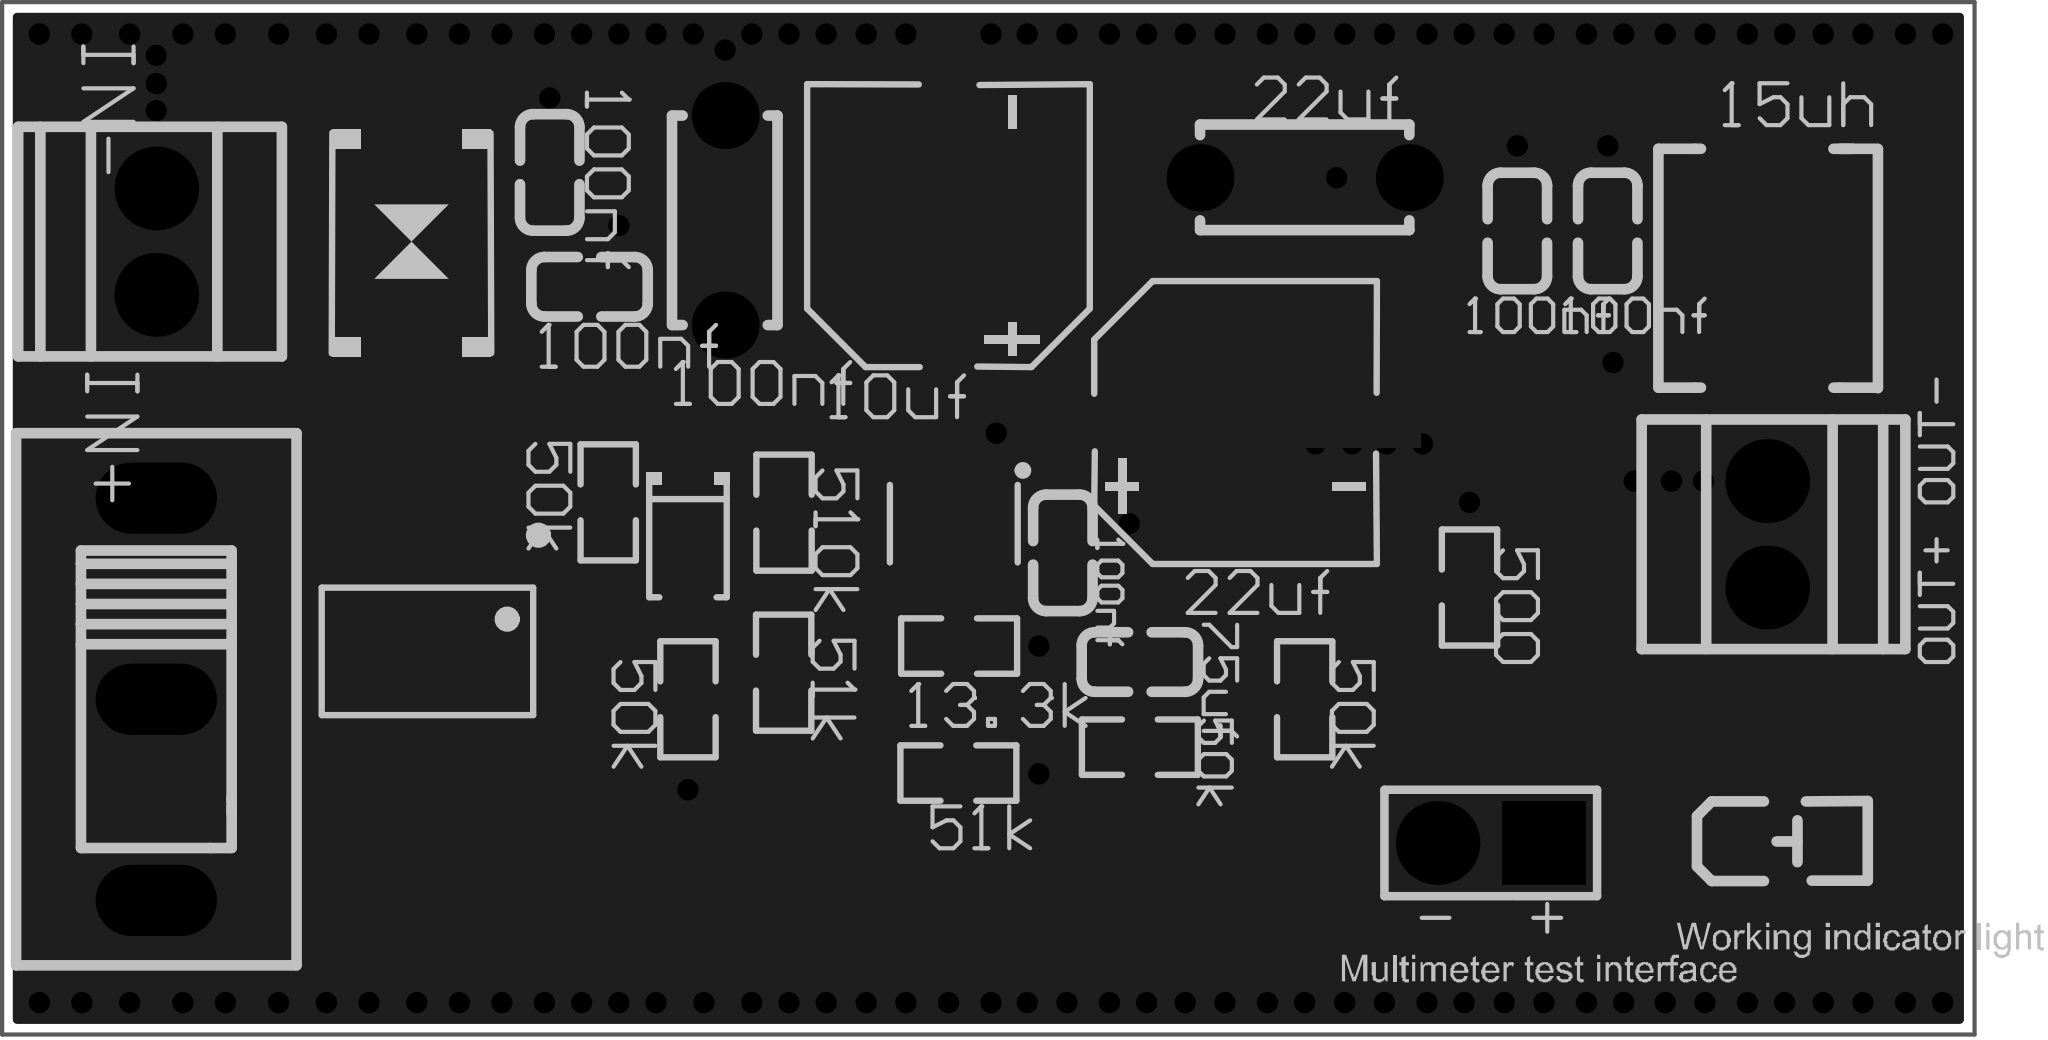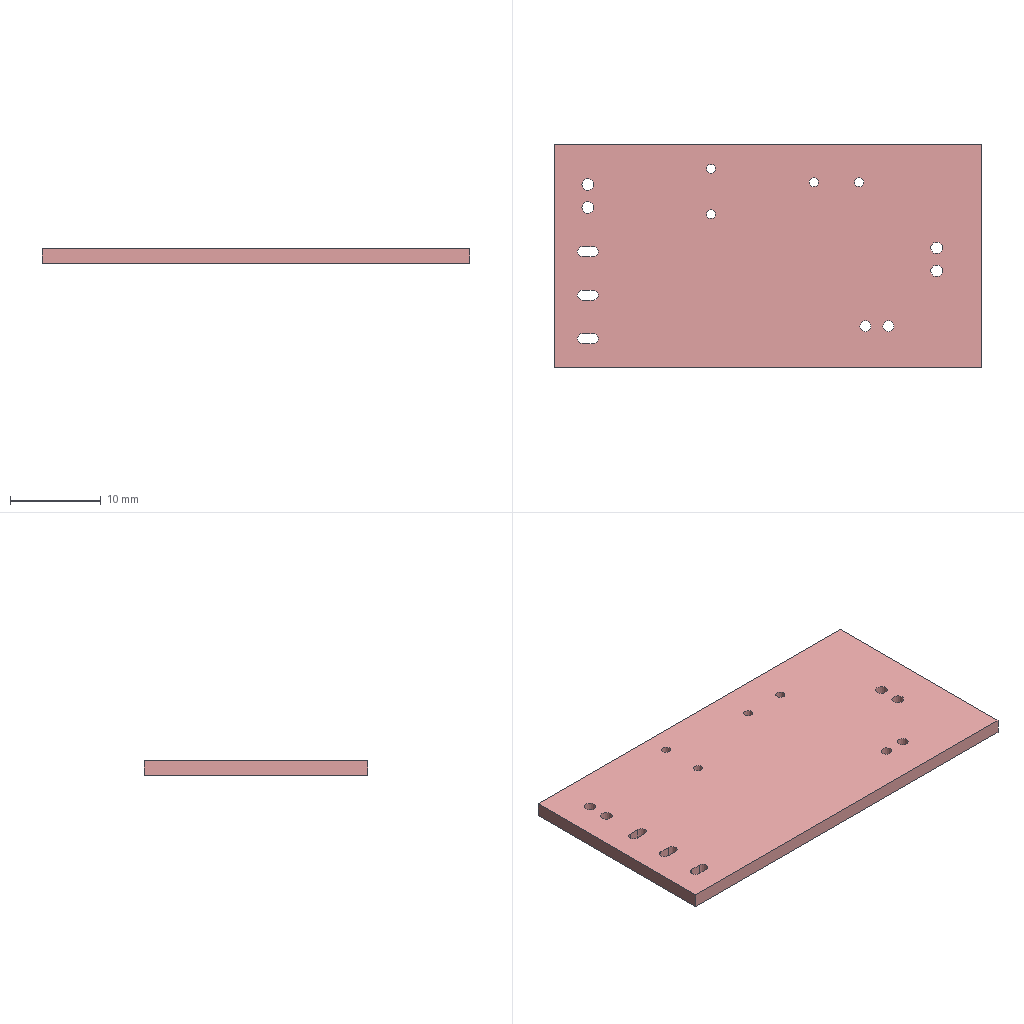Circuit board layout | Altium Designer | box 47.1 x 24.6 x 1.6 mm
Layer stack:
# Altium Designer layer stack of  (unit mm; dielectric type: 0 none, 1 core, 2 prepreg, 3 surface material)
index,name,kind,layer,copper_thickness_mm,dielectric_type,dielectric_thickness_mm,dielectric_material,dielectric_constant
0,Top Paste Mask Layer,other,,,,,,
1,Top Silkscreen Layer,other,,,,,,
2,Top Solder Mask Layer,dielectric,,,3,0.01,,3.3
3,Top Layer,copper,Top Layer,0.035,,,,
4,Dielectric1,dielectric,,,3,1.51,FR4,4.5
5,Bottom Layer,copper,Bottom Layer,0.035,,,,
6,Bottom Solder Mask Layer,dielectric,,,3,0.01,,3.3
7,Bottom Silkscreen Layer,other,,,,,,
8,Bottom Paste Mask Layer,other,,,,,,
# drill layer pairs: low layer,high layer
drill_pair,Top Layer,Bottom Layer
Part placement:
Designator,Comment,Layer,Footprint,Center-X(mm),Center-Y(mm),Rotation
C1,75uf,TopLayer,C0603,107.569,92.71,0
C5,0.1uf,TopLayer,C0603,105.729,95.315,270
C11,10uf,TopLayer,CAP-SMD_BD6.3-L6.6-W6.6-FD,102.997,103.124,90
C12,100nf,TopLayer,CAP-TH_L5.0-W2.5-P5.00-D1.0,97.663,103.251,270
C13,22uf,TopLayer,CAP-SMD_BD6.3-L6.6-W6.6-FD,109.855,98.425,0
C16,22uf,TopLayer,CAP-TH_L5.0-W2.5-P5.00-D1.0,111.506,104.267,180
D3,SMBJ28CA,TopLayer,SMB_L4.6-W3.6-LS5.4-BI,90.17,102.743,270
D4,BZT52C12,TopLayer,SOD-123_L2.7-W1.6-LS3.7-RD,96.774,95.631,270
H3,PZ254V-11-02P,TopLayer,HDR-TH_2P-P2.54-V-M,115.951,88.392,180
L1,15uH,TopLayer,IND-SMD_L5.7-W5.2_GSM0530,122.555,102.108,90
LED1,NCD0805R1,TopLayer,LED0805-RD,122.977,88.433,0
Q1,AO4421,TopLayer,SOIC-8_L4.9-W3.9-P1.27-LS6.0-BL,90.551,92.964,180
SW1,SS12D10G4 071,TopLayer,SW-TH_SHOU-HAN_SS12D10G4,84.074,91.821,270
U1,GD30DC1354,TopLayer,SOT-23-6_L2.9-W1.7-P0.95-LS2.8-BL,103.124,96.012,180
U2,KF128-2.54-2P,TopLayer,CONN-TH_P2.54_KF128-2.54-2P,122.555,95.758,90
U3,KF128-2.54-2P,TopLayer,CONN-TH_P2.54_KF128-2.54-2P,84.074,102.743,270
C21,0.1uf,TopLayer,C0603,118.745,102.997,90
C22,0.1uf,TopLayer,C0603,116.586,102.997,90
C23,100nf,TopLayer,C0603,94.423,101.665,0
C24,100nf,TopLayer,C0603,93.472,104.394,90
R7,510kΩ,TopLayer,R0603,99.069,96.275,90
R8,51kΩ,TopLayer,R0603,99.06,92.456,90
R9,500Ω,TopLayer,R0603,115.443,94.488,270
R10,50kΩ,TopLayer,R0603,107.569,90.678,0
R11,13.3kΩ,TopLayer,R0603,103.251,93.091,180
R12,50kΩ,TopLayer,R0603,111.506,91.821,90
R13,51kΩ,TopLayer,R0603,103.234,90.06,180
R15,50kΩ,TopLayer,R0603,96.774,91.821,90
R16,50kΩ,TopLayer,R0603,94.869,96.52,90
Pad and via stacks:
# Altium Designer via and pad stacks of  (unit mm). Each distinct definition once, with the count of objects using it.
# via: kind,start_layer,end_layer,hole_mm,diameter_mm,mode(0 simple;1 top-mid-bottom;2 full stack),diameter_per_layer,count,example_net
# pad: kind,layer,hole_mm,hole_type(0 round;1 square;2 slot),plating,top_size,top_shape(1 round;2 rect;3 octagon;9 rounded rect),mid_size,bottom_size,mode,footprint,size_per_layer,count,example
pad,Top Layer,0,0,plated,0.8x0.9,2,0.8x0.9,0.8x0.9,0,C0603,,12,C1.2
pad,Top Layer,0,0,plated,3.5x1.2,2,3.5x1.2,3.5x1.2,0,CAP-SMD_BD6.3-L6.6-W6.6-FD,,4,C11.1
pad,Top Layer,0,0,plated,2.047x2.241,2,2.047x2.241,2.047x2.241,0,SMB_L4.6-W3.6-LS5.4-BI,,2,D3.2
pad,Top Layer,0,0,plated,0.91x1.22,2,0.91x1.22,0.91x1.22,0,SOD-123_L2.7-W1.6-LS3.7-RD,,2,D4.2
pad,Top Layer,0,0,plated,1.5x2.7,2,1.5x2.7,1.5x2.7,0,IND-SMD_L5.7-W5.2_GSM0530,,2,L1.2
pad,Top Layer,0,0,plated,1x1.25,2,1x1.25,1x1.25,0,LED0805-RD,,2,LED1.2
pad,Top Layer,0,0,plated,0.588x2.045,1,0.588x2.045,0.588x2.045,0,SOIC-8_L4.9-W3.9-P1.27-LS6.0-BL,,8,Q1.5
pad,Top Layer,0,0,plated,0.532x0.99,2,0.532x0.99,0.532x0.99,0,SOT-23-6_L2.9-W1.7-P0.95-LS2.8-BL,,6,U1.1
pad,Top Layer,0,0,plated,0.8065x0.864,2,0.8065x0.864,0.8065x0.864,0,R0603,,18,R7.2
pad,Multi-Layer,1,0,plated,1.6x1.6,1,1.6x1.6,1.6x1.6,0,CAP-TH_L5.0-W2.5-P5.00-D1.0,,4,C12.1
pad,Multi-Layer,1.2,0,plated,2x2,2,2x2,2x2,0,HDR-TH_2P-P2.54-V-M,,1,H3.1
pad,Multi-Layer,1.2,0,plated,2x2,1,2x2,2x2,0,HDR-TH_2P-P2.54-V-M,,1,H3.2
pad,Multi-Layer,1.1,2,plated,1.7x2.9,1,1.7x2.9,1.7x2.9,0,SW-TH_SHOU-HAN_SS12D10G4,,3,SW1.1
pad,Multi-Layer,1.3,0,plated,2x2,1,2x2,2x2,0,CONN-TH_P2.54_KF128-2.54-2P,,4,U2.1
via,Top Layer,Bottom Layer,0.254,0.508,0,,126,GND
Copper pours:
name,layer,net,type(0 solid;1 hatched;2 none)
Top Layer-GND,Top Layer,GND,0
Bottom Layer-GND,Bottom Layer,GND,0
Design rules, without the lines most boards share:
# Altium Designer design rules of  (exported by Altium Designer, unit mm)
# columns: name | kind | enabled | priority | scope1 | scope2 | descriptor | typed fields (field=value)
copperThickness1oz_2 | 2 | enabled | 2 | All | All | Width Constraint (Min=5mil) (Max=100mil) (Preferred=20mil) (All) |
viaSize | 11 | enabled | 1 | All | All | Routing Via (MinHoleWidth=9mil) (MaxHoleWidth=248.031mil) (PreferredHoleWidth=10mil) (MinWidth=19.685mil) (MaxWidth=393.701mil) (PreferedWidth=20mil) (All) | via_min_hole=0.2286 via_max_hole=6.3 via_preferred_diameter=0.508 via_preferred_hole=0.254
copperRegion | 20 | enabled | 1 | All | All | Polygon Connect Rule(Direct Connect )(Conductor Width=10mil) (Relief Angle=90 Angle) (Entries=4) (Air Gap Width=10mil) (All),(All) | connect_style(0=relief,1=direct,2=none)=1 relief_conductor_width=0.254 relief_entries=4